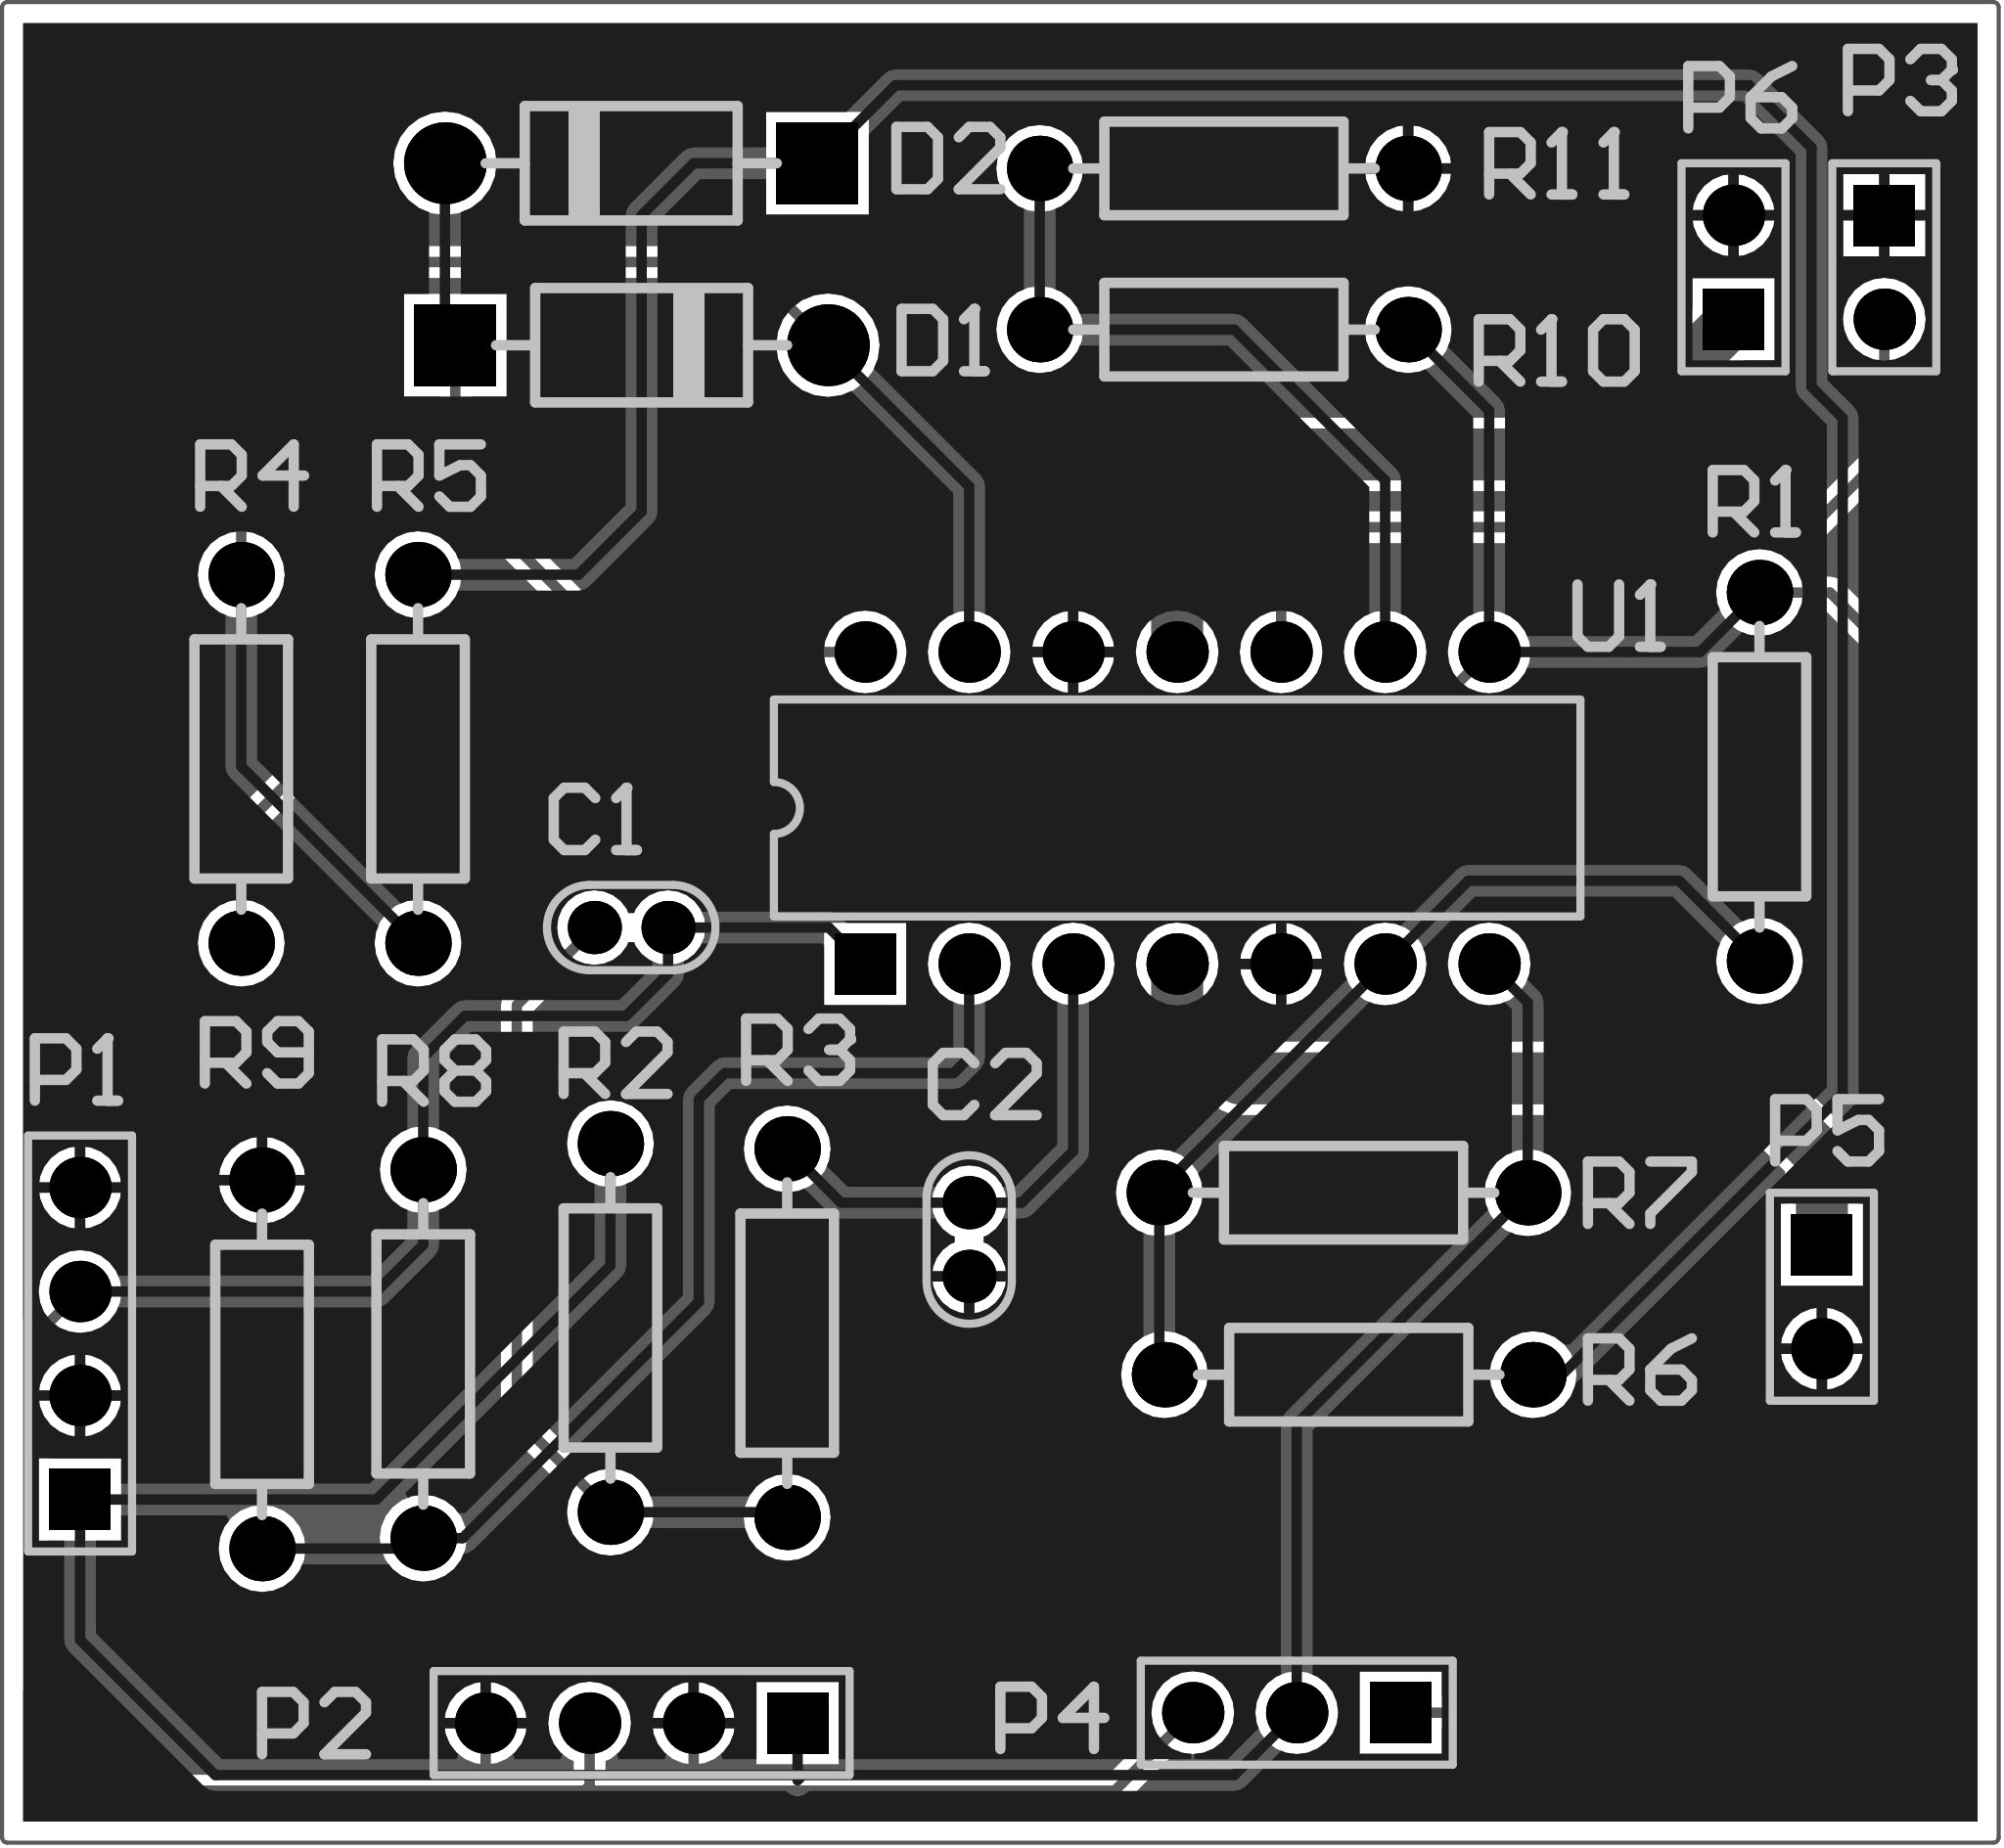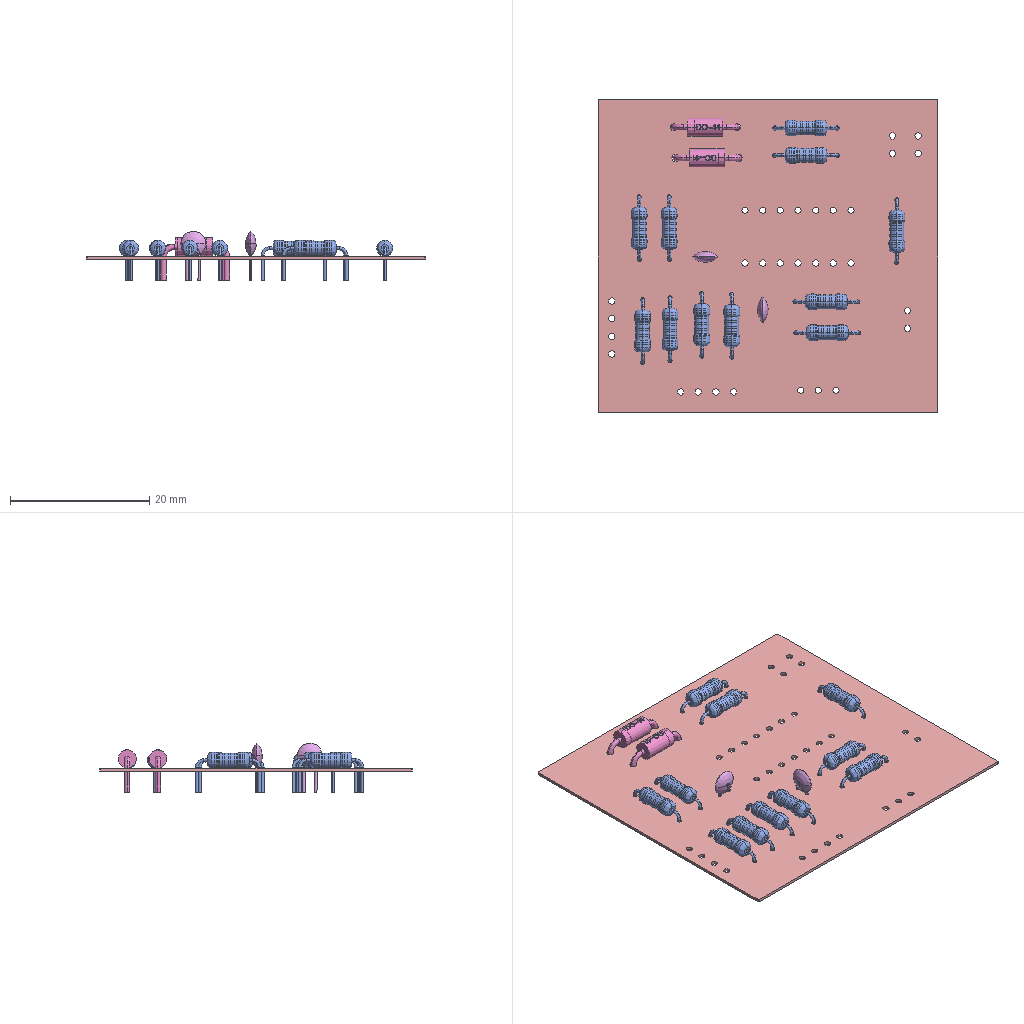Circuit board layout | Altium Designer | box 48.8 x 45 x 7.1 mm
Layer stack:
# Altium Designer layer stack of  (unit mm; dielectric type: 0 none, 1 core, 2 prepreg, 3 surface material)
index,name,kind,layer,copper_thickness_mm,dielectric_type,dielectric_thickness_mm,dielectric_material,dielectric_constant
0,Top Paste,other,,,,,,
1,Top Overlay,other,,,,,,
2,Top Solder,dielectric,,,3,0.0102,Solder Resist,3.5
3,Top Layer,copper,Top Layer,0.0356,,,,
4,Dielectric 1,dielectric,,,0,0.32,FR-4,4.8
5,Bottom Layer,copper,Bottom Layer,0.0356,,,,
6,Bottom Solder,dielectric,,,3,0.0102,Solder Resist,3.5
7,Bottom Overlay,other,,,,,,
8,Bottom Paste,other,,,,,,
# drill layer pairs: low layer,high layer
drill_pair,Top Layer,Bottom Layer
Part placement:
Designator,Comment,Layer,Footprint,Center-X(mm),Center-Y(mm),Rotation
U1,LM224N,TopLayer,646-06,104.521,54.356,360
R11,1K,TopLayer,RS_1/4W,105.664,69.977,180
R10,1K,TopLayer,RS_1/4W,105.664,66.04,360
R9,22K,TopLayer,RS_1/4W,82.169,40.767,270
R8,22K,TopLayer,RS_1/4W,86.106,41.021,90
R7,20K,TopLayer,RS_1/4W,108.585,44.958,360
R6,10K,TopLayer,RS_1/4W,108.712,40.513,180
R5,10K,TopLayer,RS_1/4W,85.979,55.554,90
R4,10K,TopLayer,RS_1/4W,81.661,55.554,90
R3,20K,TopLayer,RS_1/4W,94.996,41.529,90
R2,20K,TopLayer,RS_1/4W,90.678,41.656,270
R1,20K,TopLayer,RS_1/4W,118.745,55.118,270
P6,Header 2,TopLayer,HDR1X2,118.11,67.564,90
P5,Header 2,TopLayer,HDR1X2,120.269,42.418,270
P4,Header 3,TopLayer,HDR1X3,107.442,32.258,180
P3,Header 2,TopLayer,HDR1X2,121.793,67.564,270
P2,Header 4,TopLayer,HDR1X4,91.44,32.004,180
P1,Header 4,TopLayer,HDR1X4,77.724,41.275,90
D2,1N4007,TopLayer,DO-41,91.186,70.104,180
D1,1N4007,TopLayer,DO-41,91.44,65.659,360
C2,1UF,TopLayer,CC_1.8*3.6,99.441,43.815,270
C1,1UF,TopLayer,CC_1.8*3.6,91.186,51.435,0
Pad and via stacks:
# Altium Designer via and pad stacks of  (unit mm). Each distinct definition once, with the count of objects using it.
# via: kind,start_layer,end_layer,hole_mm,diameter_mm,mode(0 simple;1 top-mid-bottom;2 full stack),diameter_per_layer,count,example_net
# pad: kind,layer,hole_mm,hole_type(0 round;1 square;2 slot),plating,top_size,top_shape(1 round;2 rect;3 octagon;9 rounded rect),mid_size,bottom_size,mode,footprint,size_per_layer,count,example
pad,Multi-Layer,0.9,0,plated,1.5x1.5,1,1.5x1.5,1.5x1.5,0,HDR1X4,,6,P2.4
pad,Multi-Layer,0.9,0,plated,1.5x1.5,2,1.5x1.5,1.5x1.5,0,HDR1X4,,2,P2.1
pad,Multi-Layer,0.5,0,plated,1.3x1.3,1,1.3x1.3,1.3x1.3,0,CC 1.8*3.6,,4,C1.2
pad,Multi-Layer,0.6,0,plated,1.6x1.6,1,1.6x1.6,1.6x1.6,0,RS 1/4W,,22,R1.2
pad,Multi-Layer,0.9,0,plated,1.5x1.5,1,1.5x1.5,1.5x1.5,0,646-06,,13,U1.8
pad,Multi-Layer,0.9,0,plated,1.5x1.5,2,1.5x1.5,1.5x1.5,0,646-06,,1,U1.1
pad,Multi-Layer,0.9,0,plated,1.5x1.5,2,1.5x1.5,1.5x1.5,0,HDR1X2,,3,P3.1
pad,Multi-Layer,0.9,0,plated,1.5x1.5,1,1.5x1.5,1.5x1.5,0,HDR1X2,,3,P3.2
pad,Multi-Layer,1,0,plated,2x2,1,2x2,2x2,0,DO-41,,2,D1.2
pad,Multi-Layer,1,0,plated,2x2,2,2x2,2x2,0,DO-41,,2,D1.1
pad,Multi-Layer,0.9,0,plated,1.5x1.5,2,1.5x1.5,1.5x1.5,0,HDR1X3,,1,P4.1
pad,Multi-Layer,0.9,0,plated,1.5x1.5,1,1.5x1.5,1.5x1.5,0,HDR1X3,,2,P4.2
Copper pours:
name,layer,net,type(0 solid;1 hatched;2 none)
D,Top Layer,GND,0
D,Bottom Layer,GND,0
Design rules, without the lines most boards share:
# Altium Designer design rules of  (exported by Altium Designer, unit mm)
# columns: name | kind | enabled | priority | scope1 | scope2 | descriptor | typed fields (field=value)
SilkToSilkClearance | 55 | enabled | 1 | All | All | Silk to Silk (Clearance=0mil) (All),(All) |
SilkToSolderMaskClearance | 54 | enabled | 1 | IsPad | All | Silk To Solder Mask (Clearance=0mil) (IsPad),(All) |
MinimumSolderMaskSliver | 53 | enabled | 1 | All | All | Minimum Solder Mask Sliver (Gap=0mil) (All),(All) |
HoleToHoleClearance | 52 | enabled | 1 | All | All | Hole To Hole Clearance (Gap=10mil) (All),(All) | gap=0.254
DiffPairsRouting | 51 | enabled | 1 | All | All | Differential Pairs Uncoupled Length using the Gap Constraints (Min=10mil) (Max=10mil) (Prefered=10mil)  and Width Constraints (Min=15mil) (Max=15mil) (Prefered=15mil) (All) |
SolderMaskExpansion | 13 | enabled | 1 | All | All | Solder Mask Expansion (Expansion =4mil) (All) | expansion=0.1016
PasteMaskExpansion | 14 | enabled | 1 | All | All | Paste Mask Expansion (Expansion =0mil) (All) | expansion=0
RoutingVias | 11 | enabled | 1 | All | All | Routing Via (MinHoleWidth=28mil) (MaxHoleWidth=28mil) (PreferredHoleWidth=28mil) (MinWidth=50mil) (MaxWidth=50mil) (PreferedWidth=50mil) (All) | via_min_hole=0.7112 via_max_hole=0.7112 via_preferred_diameter=1.27 via_preferred_hole=0.7112
Width | 2 | enabled | 1 | All | All | Width Constraint (Min=10mil) (Max=50mil) (Preferred=10mil) (All) |
PolygonConnect | 20 | enabled | 1 | All | All | Polygon Connect Rule(Relief Connect )(Conductor Width=10mil) (Relief Angle=90 Angle) (Entries=4) (Air Gap Width=10mil) (All),(All) | connect_style(0=relief,1=direct,2=none)=0 relief_conductor_width=0.254 relief_entries=4
PlaneConnect | 6 | enabled | 1 | All | All | Power Plane Connect Rule(Relief Connect )(Expansion=20mil) (Conductor Width=10mil) (Air Gap=10mil) (Entries=4) (All) | relief_conductor_width=0.254 relief_entries=4 relief_expansion=0.508
Clearance | 0 | enabled | 1 | All | All | Clearance Constraint (Gap=10mil) (All),(All) | gap=0.254
Classes set for this board:
# Altium Designer classes of  (member kind: 0 net, 1 component, 2 from-to, 3 pad, 4 layer, 5 differential pair, 6 design channel, 7 polygon, 8 structure, 9 xSignal)
# columns: class name | member kind | superclass | members
Sheet1 | 1 | no | C1; C2; D1; D2; P1; P2; P3; P4; P5; P6; R1; R2; R3; R4; R5; R6; R7; R8; R9; R10; R11; U1;